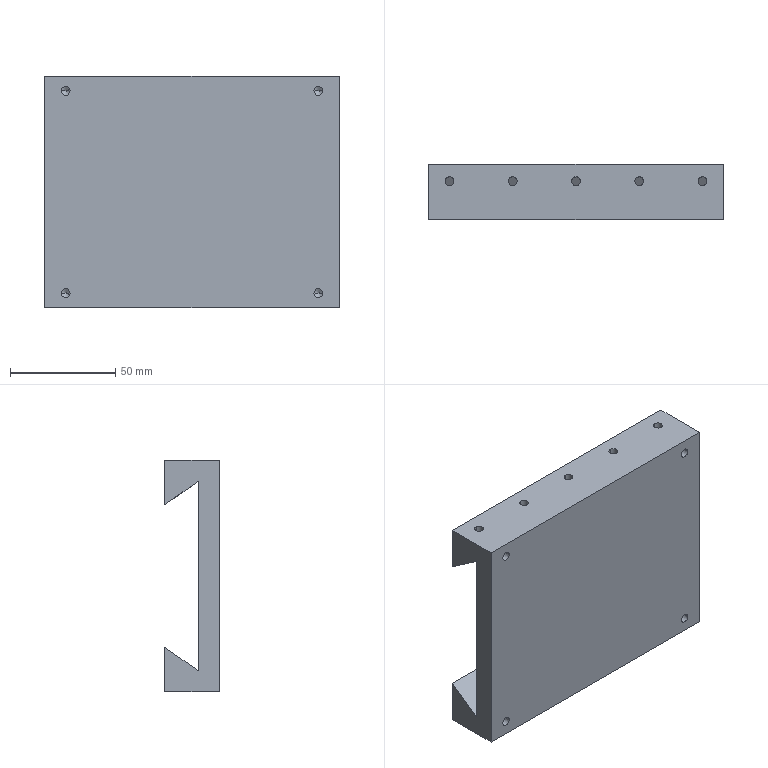Part | STEP file | 06-34 Front-rear adjusting dovetail groove | 1 solid | 36 faces | box 140 x 26 x 110 mm | volume 222237 mm3 | cylinder 18 | plane 10 | cone 8 | commonest cylinder face diameters 4.2 x18